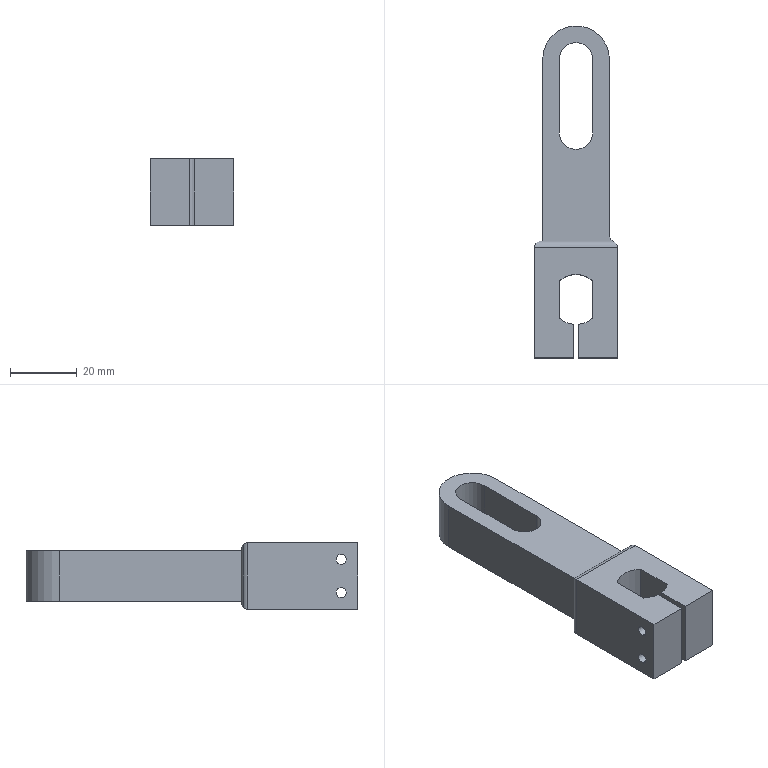Part | SolidWorks | features BaseBody 1 | 1 solid | 47 faces | box 25 x 99.5 x 20 mm | volume 28099 mm3 | cylinder 28 | plane 19 | commonest cylinder face diameters 4 x9 3 x8 6 x4 15 x3 10 x2 20 x2
STEP:
#1=CARTESIAN_POINT('',(10.5,17.5,2.));
#2=VERTEX_POINT('',#1);
#3=CARTESIAN_POINT('',(11.914,16.914,0.5858));
#4=VERTEX_POINT('',#3);
#5=CARTESIAN_POINT('',(10.5,17.5,2.));
#6=CARTESIAN_POINT('',(11.038,17.5,1.462));
#7=CARTESIAN_POINT('',(11.534,17.294,0.9659));
#8=CARTESIAN_POINT('',(11.914,16.914,0.5858));
#9=(BOUNDED_CURVE()B_SPLINE_CURVE(3,(#5,#6,#7,#8),.UNSPECIFIED.,.F.,.T.)B_SPLINE_CURVE_WITH_KNOTS((4,4),(1.571,2.356),.UNSPECIFIED.)CURVE()GEOMETRIC_REPRESENTATION_ITEM()RATIONAL_B_SPLINE_CURVE((1.,0.9493,0.9493,1.))REPRESENTATION_ITEM(''));
#10=EDGE_CURVE('',#2,#4,#9,.T.);
#11=ORIENTED_EDGE('',*,*,#10,.T.);
#12=CARTESIAN_POINT('',(-11.914,16.914,0.5858));
#13=VERTEX_POINT('',#12);
#14=CARTESIAN_POINT('',(0.,16.914,0.5858));
#15=DIRECTION('',(-1.,0.,0.));
#16=VECTOR('',#15,1000.);
#17=LINE('',#14,#16);
#18=EDGE_CURVE('',#4,#13,#17,.T.);
#19=ORIENTED_EDGE('',*,*,#18,.T.);
#20=CARTESIAN_POINT('',(-10.5,17.5,2.));
#21=VERTEX_POINT('',#20);
#22=CARTESIAN_POINT('',(-11.914,16.914,0.5858));
#23=CARTESIAN_POINT('',(-11.534,17.294,0.9659));
#24=CARTESIAN_POINT('',(-11.038,17.5,1.462));
#25=CARTESIAN_POINT('',(-10.5,17.5,2.));
#26=(BOUNDED_CURVE()B_SPLINE_CURVE(3,(#22,#23,#24,#25),.UNSPECIFIED.,.F.,.T.)B_SPLINE_CURVE_WITH_KNOTS((4,4),(0.7854,1.571),.UNSPECIFIED.)CURVE()GEOMETRIC_REPRESENTATION_ITEM()RATIONAL_B_SPLINE_CURVE((1.,0.9493,0.9493,1.))REPRESENTATION_ITEM(''));
#27=EDGE_CURVE('',#13,#21,#26,.T.);
#28=ORIENTED_EDGE('',*,*,#27,.T.);
#29=CARTESIAN_POINT('',(0.,17.5,2.));
#30=DIRECTION('',(1.,0.,0.));
#31=VECTOR('',#30,1000.);
#32=LINE('',#29,#31);
#33=EDGE_CURVE('',#21,#2,#32,.T.);
#34=ORIENTED_EDGE('',*,*,#33,.T.);
#35=EDGE_LOOP('',(#11,#19,#28,#34));
#36=FACE_OUTER_BOUND('',#35,.T.);
#37=CARTESIAN_POINT('',(0.,15.5,2.));
#38=DIRECTION('',(-1.,0.,0.));
#39=DIRECTION('',(0.,0.7071,-0.7071));
#40=AXIS2_PLACEMENT_3D('',#37,#38,#39);
#41=CYLINDRICAL_SURFACE('',#40,2.);
#42=ADVANCED_FACE('',(#36),#41,.T.);
#43=CARTESIAN_POINT('',(10.5,17.5,18.));
#44=VERTEX_POINT('',#43);
#45=CARTESIAN_POINT('',(11.914,16.914,19.414));
#46=VERTEX_POINT('',#45);
#47=CARTESIAN_POINT('',(10.5,17.5,18.));
#48=CARTESIAN_POINT('',(11.038,17.5,18.538));
#49=CARTESIAN_POINT('',(11.534,17.294,19.034));
#50=CARTESIAN_POINT('',(11.914,16.914,19.414));
#51=(BOUNDED_CURVE()B_SPLINE_CURVE(3,(#47,#48,#49,#50),.UNSPECIFIED.,.F.,.T.)B_SPLINE_CURVE_WITH_KNOTS((4,4),(1.571,2.356),.UNSPECIFIED.)CURVE()GEOMETRIC_REPRESENTATION_ITEM()RATIONAL_B_SPLINE_CURVE((1.,0.9493,0.9493,1.))REPRESENTATION_ITEM(''));
#52=EDGE_CURVE('',#44,#46,#51,.T.);
#53=ORIENTED_EDGE('',*,*,#52,.T.);
#54=CARTESIAN_POINT('',(11.914,16.914,0.));
#55=DIRECTION('',(0.,0.,-1.));
#56=VECTOR('',#55,1000.);
#57=LINE('',#54,#56);
#58=EDGE_CURVE('',#46,#4,#57,.T.);
#59=ORIENTED_EDGE('',*,*,#58,.T.);
#60=ORIENTED_EDGE('',*,*,#10,.F.);
#61=CARTESIAN_POINT('',(10.5,17.5,2.5));
#62=VERTEX_POINT('',#61);
#63=CARTESIAN_POINT('',(10.5,17.5,0.));
#64=DIRECTION('',(0.,0.,1.));
#65=VECTOR('',#64,1000.);
#66=LINE('',#63,#65);
#67=EDGE_CURVE('',#2,#62,#66,.T.);
#68=ORIENTED_EDGE('',*,*,#67,.T.);
#69=CARTESIAN_POINT('',(11.25,17.354,2.5));
#70=VERTEX_POINT('',#69);
#71=CARTESIAN_POINT('',(10.5,15.5,2.5));
#72=DIRECTION('',(0.,0.,-1.));
#73=DIRECTION('',(0.7071,0.7071,0.));
#74=AXIS2_PLACEMENT_3D('',#71,#72,#73);
#75=CIRCLE('',#74,2.);
#76=EDGE_CURVE('',#62,#70,#75,.T.);
#77=ORIENTED_EDGE('',*,*,#76,.T.);
#78=CARTESIAN_POINT('',(11.25,17.354,17.5));
#79=VERTEX_POINT('',#78);
#80=CARTESIAN_POINT('',(11.25,17.354,0.));
#81=DIRECTION('',(0.,0.,-1.));
#82=VECTOR('',#81,1000.);
#83=LINE('',#80,#82);
#84=EDGE_CURVE('',#79,#70,#83,.T.);
#85=ORIENTED_EDGE('',*,*,#84,.F.);
#86=CARTESIAN_POINT('',(10.5,17.5,17.5));
#87=VERTEX_POINT('',#86);
#88=CARTESIAN_POINT('',(10.5,15.5,17.5));
#89=DIRECTION('',(0.,0.,1.));
#90=DIRECTION('',(0.7071,0.7071,0.));
#91=AXIS2_PLACEMENT_3D('',#88,#89,#90);
#92=CIRCLE('',#91,2.);
#93=EDGE_CURVE('',#79,#87,#92,.T.);
#94=ORIENTED_EDGE('',*,*,#93,.T.);
#95=CARTESIAN_POINT('',(10.5,17.5,0.));
#96=DIRECTION('',(0.,0.,1.));
#97=VECTOR('',#96,1000.);
#98=LINE('',#95,#97);
#99=EDGE_CURVE('',#87,#44,#98,.T.);
#100=ORIENTED_EDGE('',*,*,#99,.T.);
#101=EDGE_LOOP('',(#53,#59,#60,#68,#77,#85,#94,#100));
#102=FACE_OUTER_BOUND('',#101,.T.);
#103=CARTESIAN_POINT('',(10.5,15.5,0.));
#104=DIRECTION('',(0.,0.,-1.));
#105=DIRECTION('',(0.7071,0.7071,0.));
#106=AXIS2_PLACEMENT_3D('',#103,#104,#105);
#107=CYLINDRICAL_SURFACE('',#106,2.);
#108=ADVANCED_FACE('',(#102),#107,.T.);
#109=CARTESIAN_POINT('',(-11.914,16.914,19.414));
#110=VERTEX_POINT('',#109);
#111=CARTESIAN_POINT('',(-10.5,17.5,18.));
#112=VERTEX_POINT('',#111);
#113=CARTESIAN_POINT('',(-11.914,16.914,19.414));
#114=CARTESIAN_POINT('',(-11.534,17.294,19.034));
#115=CARTESIAN_POINT('',(-11.038,17.5,18.538));
#116=CARTESIAN_POINT('',(-10.5,17.5,18.));
#117=(BOUNDED_CURVE()B_SPLINE_CURVE(3,(#113,#114,#115,#116),.UNSPECIFIED.,.F.,.T.)B_SPLINE_CURVE_WITH_KNOTS((4,4),(3.927,4.712),.UNSPECIFIED.)CURVE()GEOMETRIC_REPRESENTATION_ITEM()RATIONAL_B_SPLINE_CURVE((1.,0.9493,0.9493,1.))REPRESENTATION_ITEM(''));
#118=EDGE_CURVE('',#110,#112,#117,.T.);
#119=ORIENTED_EDGE('',*,*,#118,.F.);
#120=CARTESIAN_POINT('',(-0.9115,16.914,19.414));
#121=DIRECTION('',(1.,0.,0.));
#122=VECTOR('',#121,1000.);
#123=LINE('',#120,#122);
#124=EDGE_CURVE('',#110,#46,#123,.T.);
#125=ORIENTED_EDGE('',*,*,#124,.T.);
#126=ORIENTED_EDGE('',*,*,#52,.F.);
#127=CARTESIAN_POINT('',(-0.9115,17.5,18.));
#128=DIRECTION('',(-1.,0.,0.));
#129=VECTOR('',#128,1000.);
#130=LINE('',#127,#129);
#131=EDGE_CURVE('',#44,#112,#130,.T.);
#132=ORIENTED_EDGE('',*,*,#131,.T.);
#133=EDGE_LOOP('',(#119,#125,#126,#132));
#134=FACE_OUTER_BOUND('',#133,.T.);
#135=CARTESIAN_POINT('',(-0.9115,15.5,18.));
#136=DIRECTION('',(1.,0.,0.));
#137=DIRECTION('',(0.,0.7071,0.7071));
#138=AXIS2_PLACEMENT_3D('',#135,#136,#137);
#139=CYLINDRICAL_SURFACE('',#138,2.);
#140=ADVANCED_FACE('',(#134),#139,.T.);
#141=CARTESIAN_POINT('',(-12.5,15.5,20.));
#142=VERTEX_POINT('',#141);
#143=CARTESIAN_POINT('',(-12.5,15.5,20.));
#144=CARTESIAN_POINT('',(-12.5,16.038,20.));
#145=CARTESIAN_POINT('',(-12.294,16.534,19.794));
#146=CARTESIAN_POINT('',(-11.914,16.914,19.414));
#147=(BOUNDED_CURVE()B_SPLINE_CURVE(3,(#143,#144,#145,#146),.UNSPECIFIED.,.F.,.T.)B_SPLINE_CURVE_WITH_KNOTS((4,4),(3.142,3.927),.UNSPECIFIED.)CURVE()GEOMETRIC_REPRESENTATION_ITEM()RATIONAL_B_SPLINE_CURVE((1.,0.9493,0.9493,1.))REPRESENTATION_ITEM(''));
#148=EDGE_CURVE('',#142,#110,#147,.T.);
#149=ORIENTED_EDGE('',*,*,#148,.T.);
#150=CARTESIAN_POINT('',(-11.914,16.914,0.));
#151=DIRECTION('',(0.,0.,-1.));
#152=VECTOR('',#151,1000.);
#153=LINE('',#150,#152);
#154=EDGE_CURVE('',#110,#13,#153,.T.);
#155=ORIENTED_EDGE('',*,*,#154,.T.);
#156=CARTESIAN_POINT('',(-12.5,15.5,0.));
#157=VERTEX_POINT('',#156);
#158=CARTESIAN_POINT('',(-12.5,15.5,0.));
#159=CARTESIAN_POINT('',(-12.5,16.038,0.));
#160=CARTESIAN_POINT('',(-12.294,16.534,0.2057));
#161=CARTESIAN_POINT('',(-11.914,16.914,0.5858));
#162=(BOUNDED_CURVE()B_SPLINE_CURVE(3,(#158,#159,#160,#161),.UNSPECIFIED.,.F.,.T.)B_SPLINE_CURVE_WITH_KNOTS((4,4),(0.,0.7854),.UNSPECIFIED.)CURVE()GEOMETRIC_REPRESENTATION_ITEM()RATIONAL_B_SPLINE_CURVE((1.,0.9493,0.9493,1.))REPRESENTATION_ITEM(''));
#163=EDGE_CURVE('',#157,#13,#162,.T.);
#164=ORIENTED_EDGE('',*,*,#163,.F.);
#165=CARTESIAN_POINT('',(-12.5,15.5,0.));
#166=DIRECTION('',(0.,0.,1.));
#167=VECTOR('',#166,1000.);
#168=LINE('',#165,#167);
#169=EDGE_CURVE('',#157,#142,#168,.T.);
#170=ORIENTED_EDGE('',*,*,#169,.T.);
#171=EDGE_LOOP('',(#149,#155,#164,#170));
#172=FACE_OUTER_BOUND('',#171,.T.);
#173=CARTESIAN_POINT('',(-10.5,15.5,0.));
#174=DIRECTION('',(0.,0.,-1.));
#175=DIRECTION('',(-0.7071,0.7071,0.));
#176=AXIS2_PLACEMENT_3D('',#173,#174,#175);
#177=CYLINDRICAL_SURFACE('',#176,2.);
#178=ADVANCED_FACE('',(#172),#177,.T.);
#179=CARTESIAN_POINT('',(-10.,72.,17.5));
#180=VERTEX_POINT('',#179);
#181=CARTESIAN_POINT('',(7.071,79.071,17.5));
#182=VERTEX_POINT('',#181);
#183=CARTESIAN_POINT('',(0.,72.,17.5));
#184=DIRECTION('',(0.,0.,-1.));
#185=DIRECTION('',(0.7071,0.7071,0.));
#186=AXIS2_PLACEMENT_3D('',#183,#184,#185);
#187=CIRCLE('',#186,10.);
#188=EDGE_CURVE('',#180,#182,#187,.T.);
#189=ORIENTED_EDGE('',*,*,#188,.T.);
#190=CARTESIAN_POINT('',(7.071,79.071,2.5));
#191=VERTEX_POINT('',#190);
#192=CARTESIAN_POINT('',(7.071,79.071,0.));
#193=DIRECTION('',(0.,0.,-1.));
#194=VECTOR('',#193,1000.);
#195=LINE('',#192,#194);
#196=EDGE_CURVE('',#182,#191,#195,.T.);
#197=ORIENTED_EDGE('',*,*,#196,.T.);
#198=CARTESIAN_POINT('',(-10.,72.,2.5));
#199=VERTEX_POINT('',#198);
#200=CARTESIAN_POINT('',(0.,72.,2.5));
#201=DIRECTION('',(0.,0.,1.));
#202=DIRECTION('',(-0.7071,0.7071,0.));
#203=AXIS2_PLACEMENT_3D('',#200,#201,#202);
#204=CIRCLE('',#203,10.);
#205=EDGE_CURVE('',#191,#199,#204,.T.);
#206=ORIENTED_EDGE('',*,*,#205,.T.);
#207=CARTESIAN_POINT('',(-10.,72.,0.));
#208=DIRECTION('',(0.,0.,1.));
#209=VECTOR('',#208,1000.);
#210=LINE('',#207,#209);
#211=EDGE_CURVE('',#199,#180,#210,.T.);
#212=ORIENTED_EDGE('',*,*,#211,.T.);
#213=EDGE_LOOP('',(#189,#197,#206,#212));
#214=FACE_OUTER_BOUND('',#213,.T.);
#215=CARTESIAN_POINT('',(0.,72.,0.));
#216=DIRECTION('',(0.,0.,-1.));
#217=DIRECTION('',(0.7071,0.7071,0.));
#218=AXIS2_PLACEMENT_3D('',#215,#216,#217);
#219=CYLINDRICAL_SURFACE('',#218,10.);
#220=ADVANCED_FACE('',(#214),#219,.T.);
#221=CARTESIAN_POINT('',(8.5,-12.5,8.));
#222=VERTEX_POINT('',#221);
#223=CARTESIAN_POINT('',(8.5,-12.5,2.));
#224=VERTEX_POINT('',#223);
#225=CARTESIAN_POINT('',(8.5,-12.5,5.));
#226=DIRECTION('',(-1.,0.,0.));
#227=DIRECTION('',(0.,0.,1.));
#228=AXIS2_PLACEMENT_3D('',#225,#226,#227);
#229=CIRCLE('',#228,3.);
#230=EDGE_CURVE('',#222,#224,#229,.T.);
#231=ORIENTED_EDGE('',*,*,#230,.T.);
#232=CARTESIAN_POINT('',(12.5,-12.5,2.));
#233=VERTEX_POINT('',#232);
#234=CARTESIAN_POINT('',(12.5,-12.5,2.));
#235=DIRECTION('',(1.,0.,0.));
#236=VECTOR('',#235,1000.);
#237=LINE('',#234,#236);
#238=EDGE_CURVE('',#224,#233,#237,.T.);
#239=ORIENTED_EDGE('',*,*,#238,.T.);
#240=CARTESIAN_POINT('',(12.5,-12.5,8.));
#241=VERTEX_POINT('',#240);
#242=CARTESIAN_POINT('',(12.5,-12.5,5.));
#243=DIRECTION('',(-1.,0.,0.));
#244=DIRECTION('',(0.,0.,1.));
#245=AXIS2_PLACEMENT_3D('',#242,#243,#244);
#246=CIRCLE('',#245,3.);
#247=EDGE_CURVE('',#241,#233,#246,.T.);
#248=ORIENTED_EDGE('',*,*,#247,.F.);
#249=CARTESIAN_POINT('',(12.5,-12.5,8.));
#250=DIRECTION('',(1.,0.,0.));
#251=VECTOR('',#250,1000.);
#252=LINE('',#249,#251);
#253=EDGE_CURVE('',#222,#241,#252,.T.);
#254=ORIENTED_EDGE('',*,*,#253,.F.);
#255=EDGE_LOOP('',(#231,#239,#248,#254));
#256=FACE_OUTER_BOUND('',#255,.T.);
#257=CARTESIAN_POINT('',(12.5,-12.5,5.));
#258=DIRECTION('',(1.,0.,0.));
#259=DIRECTION('',(0.,0.,1.));
#260=AXIS2_PLACEMENT_3D('',#257,#258,#259);
#261=CYLINDRICAL_SURFACE('',#260,3.);
#262=ADVANCED_FACE('',(#256),#261,.F.);
#263=CARTESIAN_POINT('',(8.5,-12.5,18.));
#264=VERTEX_POINT('',#263);
#265=CARTESIAN_POINT('',(8.5,-12.5,12.));
#266=VERTEX_POINT('',#265);
#267=CARTESIAN_POINT('',(8.5,-12.5,15.));
#268=DIRECTION('',(-1.,0.,0.));
#269=DIRECTION('',(0.,0.,1.));
#270=AXIS2_PLACEMENT_3D('',#267,#268,#269);
#271=CIRCLE('',#270,3.);
#272=EDGE_CURVE('',#264,#266,#271,.T.);
#273=ORIENTED_EDGE('',*,*,#272,.T.);
#274=CARTESIAN_POINT('',(12.5,-12.5,12.));
#275=VERTEX_POINT('',#274);
#276=CARTESIAN_POINT('',(12.5,-12.5,12.));
#277=DIRECTION('',(1.,0.,0.));
#278=VECTOR('',#277,1000.);
#279=LINE('',#276,#278);
#280=EDGE_CURVE('',#266,#275,#279,.T.);
#281=ORIENTED_EDGE('',*,*,#280,.T.);
#282=CARTESIAN_POINT('',(12.5,-12.5,18.));
#283=VERTEX_POINT('',#282);
#284=CARTESIAN_POINT('',(12.5,-12.5,15.));
#285=DIRECTION('',(-1.,0.,0.));
#286=DIRECTION('',(0.,0.,1.));
#287=AXIS2_PLACEMENT_3D('',#284,#285,#286);
#288=CIRCLE('',#287,3.);
#289=EDGE_CURVE('',#283,#275,#288,.T.);
#290=ORIENTED_EDGE('',*,*,#289,.F.);
#291=CARTESIAN_POINT('',(12.5,-12.5,18.));
#292=DIRECTION('',(1.,0.,0.));
#293=VECTOR('',#292,1000.);
#294=LINE('',#291,#293);
#295=EDGE_CURVE('',#264,#283,#294,.T.);
#296=ORIENTED_EDGE('',*,*,#295,.F.);
#297=EDGE_LOOP('',(#273,#281,#290,#296));
#298=FACE_OUTER_BOUND('',#297,.T.);
#299=CARTESIAN_POINT('',(12.5,-12.5,15.));
#300=DIRECTION('',(1.,0.,0.));
#301=DIRECTION('',(0.,0.,1.));
#302=AXIS2_PLACEMENT_3D('',#299,#300,#301);
#303=CYLINDRICAL_SURFACE('',#302,3.);
#304=ADVANCED_FACE('',(#298),#303,.F.);
#305=CARTESIAN_POINT('',(8.5,-12.5,3.5));
#306=VERTEX_POINT('',#305);
#307=CARTESIAN_POINT('',(8.5,-12.5,6.5));
#308=VERTEX_POINT('',#307);
#309=CARTESIAN_POINT('',(8.5,-12.5,5.));
#310=DIRECTION('',(1.,0.,0.));
#311=DIRECTION('',(0.,0.,-1.));
#312=AXIS2_PLACEMENT_3D('',#309,#310,#311);
#313=CIRCLE('',#312,1.5);
#314=EDGE_CURVE('',#306,#308,#313,.T.);
#315=ORIENTED_EDGE('',*,*,#314,.T.);
#316=CARTESIAN_POINT('',(0.75,-12.5,6.5));
#317=VERTEX_POINT('',#316);
#318=CARTESIAN_POINT('',(-12.5,-12.5,6.5));
#319=DIRECTION('',(-1.,0.,0.));
#320=VECTOR('',#319,1000.);
#321=LINE('',#318,#320);
#322=EDGE_CURVE('',#308,#317,#321,.T.);
#323=ORIENTED_EDGE('',*,*,#322,.T.);
#324=CARTESIAN_POINT('',(0.75,-12.5,3.5));
#325=VERTEX_POINT('',#324);
#326=CARTESIAN_POINT('',(0.75,-12.5,5.));
#327=DIRECTION('',(1.,0.,0.));
#328=DIRECTION('',(0.,0.,-1.));
#329=AXIS2_PLACEMENT_3D('',#326,#327,#328);
#330=CIRCLE('',#329,1.5);
#331=EDGE_CURVE('',#325,#317,#330,.T.);
#332=ORIENTED_EDGE('',*,*,#331,.F.);
#333=CARTESIAN_POINT('',(-12.5,-12.5,3.5));
#334=DIRECTION('',(-1.,0.,0.));
#335=VECTOR('',#334,1000.);
#336=LINE('',#333,#335);
#337=EDGE_CURVE('',#306,#325,#336,.T.);
#338=ORIENTED_EDGE('',*,*,#337,.F.);
#339=EDGE_LOOP('',(#315,#323,#332,#338));
#340=FACE_OUTER_BOUND('',#339,.T.);
#341=CARTESIAN_POINT('',(-12.5,-12.5,5.));
#342=DIRECTION('',(-1.,0.,0.));
#343=DIRECTION('',(0.,0.,-1.));
#344=AXIS2_PLACEMENT_3D('',#341,#342,#343);
#345=CYLINDRICAL_SURFACE('',#344,1.5);
#346=ADVANCED_FACE('',(#340),#345,.F.);
#347=CARTESIAN_POINT('',(-0.75,-12.5,6.5));
#348=VERTEX_POINT('',#347);
#349=CARTESIAN_POINT('',(-0.75,-12.5,3.5));
#350=VERTEX_POINT('',#349);
#351=CARTESIAN_POINT('',(-0.75,-12.5,5.));
#352=DIRECTION('',(-1.,0.,0.));
#353=DIRECTION('',(0.,0.,-1.));
#354=AXIS2_PLACEMENT_3D('',#351,#352,#353);
#355=CIRCLE('',#354,1.5);
#356=EDGE_CURVE('',#348,#350,#355,.T.);
#357=ORIENTED_EDGE('',*,*,#356,.F.);
#358=CARTESIAN_POINT('',(-12.5,-12.5,6.5));
#359=VERTEX_POINT('',#358);
#360=CARTESIAN_POINT('',(-12.5,-12.5,6.5));
#361=DIRECTION('',(-1.,0.,0.));
#362=VECTOR('',#361,1000.);
#363=LINE('',#360,#362);
#364=EDGE_CURVE('',#348,#359,#363,.T.);
#365=ORIENTED_EDGE('',*,*,#364,.T.);
#366=CARTESIAN_POINT('',(-12.5,-12.5,3.5));
#367=VERTEX_POINT('',#366);
#368=CARTESIAN_POINT('',(-12.5,-12.5,5.));
#369=DIRECTION('',(1.,0.,0.));
#370=DIRECTION('',(0.,0.,-1.));
#371=AXIS2_PLACEMENT_3D('',#368,#369,#370);
#372=CIRCLE('',#371,1.5);
#373=EDGE_CURVE('',#367,#359,#372,.T.);
#374=ORIENTED_EDGE('',*,*,#373,.F.);
#375=CARTESIAN_POINT('',(-12.5,-12.5,3.5));
#376=DIRECTION('',(-1.,0.,0.));
#377=VECTOR('',#376,1000.);
#378=LINE('',#375,#377);
#379=EDGE_CURVE('',#350,#367,#378,.T.);
#380=ORIENTED_EDGE('',*,*,#379,.F.);
#381=EDGE_LOOP('',(#357,#365,#374,#380));
#382=FACE_OUTER_BOUND('',#381,.T.);
#383=CARTESIAN_POINT('',(-12.5,-12.5,5.));
#384=DIRECTION('',(-1.,0.,0.));
#385=DIRECTION('',(0.,0.,-1.));
#386=AXIS2_PLACEMENT_3D('',#383,#384,#385);
#387=CYLINDRICAL_SURFACE('',#386,1.5);
#388=ADVANCED_FACE('',(#382),#387,.F.);
#389=CARTESIAN_POINT('',(8.5,-12.5,13.5));
#390=VERTEX_POINT('',#389);
#391=CARTESIAN_POINT('',(8.5,-12.5,16.5));
#392=VERTEX_POINT('',#391);
#393=CARTESIAN_POINT('',(8.5,-12.5,15.));
#394=DIRECTION('',(1.,0.,0.));
#395=DIRECTION('',(0.,0.,-1.));
#396=AXIS2_PLACEMENT_3D('',#393,#394,#395);
#397=CIRCLE('',#396,1.5);
#398=EDGE_CURVE('',#390,#392,#397,.T.);
#399=ORIENTED_EDGE('',*,*,#398,.T.);
#400=CARTESIAN_POINT('',(0.75,-12.5,16.5));
#401=VERTEX_POINT('',#400);
#402=CARTESIAN_POINT('',(-12.5,-12.5,16.5));
#403=DIRECTION('',(-1.,0.,0.));
#404=VECTOR('',#403,1000.);
#405=LINE('',#402,#404);
#406=EDGE_CURVE('',#392,#401,#405,.T.);
#407=ORIENTED_EDGE('',*,*,#406,.T.);
#408=CARTESIAN_POINT('',(0.75,-12.5,13.5));
#409=VERTEX_POINT('',#408);
#410=CARTESIAN_POINT('',(0.75,-12.5,15.));
#411=DIRECTION('',(1.,0.,0.));
#412=DIRECTION('',(0.,0.,-1.));
#413=AXIS2_PLACEMENT_3D('',#410,#411,#412);
#414=CIRCLE('',#413,1.5);
#415=EDGE_CURVE('',#409,#401,#414,.T.);
#416=ORIENTED_EDGE('',*,*,#415,.F.);
#417=CARTESIAN_POINT('',(-12.5,-12.5,13.5));
#418=DIRECTION('',(-1.,0.,0.));
#419=VECTOR('',#418,1000.);
#420=LINE('',#417,#419);
#421=EDGE_CURVE('',#390,#409,#420,.T.);
#422=ORIENTED_EDGE('',*,*,#421,.F.);
#423=EDGE_LOOP('',(#399,#407,#416,#422));
#424=FACE_OUTER_BOUND('',#423,.T.);
#425=CARTESIAN_POINT('',(-12.5,-12.5,15.));
#426=DIRECTION('',(-1.,0.,0.));
#427=DIRECTION('',(0.,0.,-1.));
#428=AXIS2_PLACEMENT_3D('',#425,#426,#427);
#429=CYLINDRICAL_SURFACE('',#428,1.5);
#430=ADVANCED_FACE('',(#424),#429,.F.);
#431=CARTESIAN_POINT('',(-0.75,-12.5,16.5));
#432=VERTEX_POINT('',#431);
#433=CARTESIAN_POINT('',(-0.75,-12.5,13.5));
#434=VERTEX_POINT('',#433);
#435=CARTESIAN_POINT('',(-0.75,-12.5,15.));
#436=DIRECTION('',(-1.,0.,0.));
#437=DIRECTION('',(0.,0.,-1.));
#438=AXIS2_PLACEMENT_3D('',#435,#436,#437);
#439=CIRCLE('',#438,1.5);
#440=EDGE_CURVE('',#432,#434,#439,.T.);
#441=ORIENTED_EDGE('',*,*,#440,.F.);
#442=CARTESIAN_POINT('',(-12.5,-12.5,16.5));
#443=VERTEX_POINT('',#442);
#444=CARTESIAN_POINT('',(-12.5,-12.5,16.5));
#445=DIRECTION('',(-1.,0.,0.));
#446=VECTOR('',#445,1000.);
#447=LINE('',#444,#446);
#448=EDGE_CURVE('',#432,#443,#447,.T.);
#449=ORIENTED_EDGE('',*,*,#448,.T.);
#450=CARTESIAN_POINT('',(-12.5,-12.5,13.5));
#451=VERTEX_POINT('',#450);
#452=CARTESIAN_POINT('',(-12.5,-12.5,15.));
#453=DIRECTION('',(1.,0.,0.));
#454=DIRECTION('',(0.,0.,-1.));
#455=AXIS2_PLACEMENT_3D('',#452,#453,#454);
#456=CIRCLE('',#455,1.5);
#457=EDGE_CURVE('',#451,#443,#456,.T.);
#458=ORIENTED_EDGE('',*,*,#457,.F.);
#459=CARTESIAN_POINT('',(-12.5,-12.5,13.5));
#460=DIRECTION('',(-1.,0.,0.));
#461=VECTOR('',#460,1000.);
#462=LINE('',#459,#461);
#463=EDGE_CURVE('',#434,#451,#462,.T.);
#464=ORIENTED_EDGE('',*,*,#463,.F.);
#465=EDGE_LOOP('',(#441,#449,#458,#464));
#466=FACE_OUTER_BOUND('',#465,.T.);
#467=CARTESIAN_POINT('',(-12.5,-12.5,15.));
#468=DIRECTION('',(-1.,0.,0.));
#469=DIRECTION('',(0.,0.,-1.));
#470=AXIS2_PLACEMENT_3D('',#467,#468,#469);
#471=CYLINDRICAL_SURFACE('',#470,1.5);
#472=ADVANCED_FACE('',(#466),#471,.F.);
#473=CARTESIAN_POINT('',(10.,19.208,17.5));
#474=VERTEX_POINT('',#473);
#475=CARTESIAN_POINT('',(12.,19.208,17.5));
#476=DIRECTION('',(0.,0.,-1.));
#477=DIRECTION('',(1.,0.,0.));
#478=AXIS2_PLACEMENT_3D('',#475,#476,#477);
#479=CIRCLE('',#478,2.);
#480=EDGE_CURVE('',#79,#474,#479,.T.);
#481=ORIENTED_EDGE('',*,*,#480,.F.);
#482=ORIENTED_EDGE('',*,*,#84,.T.);
#483=CARTESIAN_POINT('',(10.,19.208,2.5));
#484=VERTEX_POINT('',#483);
#485=CARTESIAN_POINT('',(12.,19.208,2.5));
#486=DIRECTION('',(0.,0.,-1.));
#487=DIRECTION('',(1.,0.,0.));
#488=AXIS2_PLACEMENT_3D('',#485,#486,#487);
#489=CIRCLE('',#488,2.);
#490=EDGE_CURVE('',#70,#484,#489,.T.);
#491=ORIENTED_EDGE('',*,*,#490,.T.);
#492=CARTESIAN_POINT('',(10.,19.208,0.));
#493=DIRECTION('',(0.,0.,1.));
#494=VECTOR('',#493,1000.);
#495=LINE('',#492,#494);
#496=EDGE_CURVE('',#484,#474,#495,.T.);
#497=ORIENTED_EDGE('',*,*,#496,.T.);
#498=EDGE_LOOP('',(#481,#482,#491,#497));
#499=FACE_OUTER_BOUND('',#498,.T.);
#500=CARTESIAN_POINT('',(12.,19.208,0.));
#501=DIRECTION('',(0.,0.,-1.));
#502=DIRECTION('',(1.,0.,0.));
#503=AXIS2_PLACEMENT_3D('',#500,#501,#502);
#504=CYLINDRICAL_SURFACE('',#503,2.);
#505=ADVANCED_FACE('',(#499),#504,.F.);
#506=ORIENTED_EDGE('',*,*,#496,.F.);
#507=CARTESIAN_POINT('',(10.,72.,2.5));
#508=VERTEX_POINT('',#507);
#509=CARTESIAN_POINT('',(10.,17.5,2.5));
#510=DIRECTION('',(0.,1.,0.));
#511=VECTOR('',#510,1000.);
#512=LINE('',#509,#511);
#513=EDGE_CURVE('',#484,#508,#512,.T.);
#514=ORIENTED_EDGE('',*,*,#513,.T.);
#515=CARTESIAN_POINT('',(10.,72.,17.5));
#516=VERTEX_POINT('',#515);
#517=CARTESIAN_POINT('',(10.,72.,0.));
#518=DIRECTION('',(0.,0.,-1.));
#519=VECTOR('',#518,1000.);
#520=LINE('',#517,#519);
#521=EDGE_CURVE('',#516,#508,#520,.T.);
#522=ORIENTED_EDGE('',*,*,#521,.F.);
#523=CARTESIAN_POINT('',(10.,49.75,17.5));
#524=DIRECTION('',(0.,-1.,0.));
#525=VECTOR('',#524,1000.);
#526=LINE('',#523,#525);
#527=EDGE_CURVE('',#516,#474,#526,.T.);
#528=ORIENTED_EDGE('',*,*,#527,.T.);
#529=EDGE_LOOP('',(#506,#514,#522,#528));
#530=FACE_OUTER_BOUND('',#529,.T.);
#531=CARTESIAN_POINT('',(10.,17.5,0.));
#532=DIRECTION('',(1.,0.,0.));
#533=DIRECTION('',(0.,1.,0.));
#534=AXIS2_PLACEMENT_3D('',#531,#532,#533);
#535=PLANE('',#534);
#536=ADVANCED_FACE('',(#530),#535,.T.);
#537=ORIENTED_EDGE('',*,*,#457,.T.);
#538=CARTESIAN_POINT('',(-12.5,-12.5,15.));
#539=DIRECTION('',(1.,0.,0.));
#540=DIRECTION('',(0.,0.,-1.));
#541=AXIS2_PLACEMENT_3D('',#538,#539,#540);
#542=CIRCLE('',#541,1.5);
#543=EDGE_CURVE('',#443,#451,#542,.T.);
#544=ORIENTED_EDGE('',*,*,#543,.T.);
#545=EDGE_LOOP('',(#537,#544));
#546=FACE_BOUND('',#545,.T.);
#547=ORIENTED_EDGE('',*,*,#373,.T.);
#548=CARTESIAN_POINT('',(-12.5,-12.5,5.));
#549=DIRECTION('',(1.,0.,0.));
#550=DIRECTION('',(0.,0.,-1.));
#551=AXIS2_PLACEMENT_3D('',#548,#549,#550);
#552=CIRCLE('',#551,1.5);
#553=EDGE_CURVE('',#359,#367,#552,.T.);
#554=ORIENTED_EDGE('',*,*,#553,.T.);
#555=EDGE_LOOP('',(#547,#554));
#556=FACE_BOUND('',#555,.T.);
#557=ORIENTED_EDGE('',*,*,#169,.F.);
#558=CARTESIAN_POINT('',(-12.5,-17.5,0.));
#559=VERTEX_POINT('',#558);
#560=CARTESIAN_POINT('',(-12.5,17.5,0.));
#561=DIRECTION('',(0.,-1.,0.));
#562=VECTOR('',#561,1000.);
#563=LINE('',#560,#562);
#564=EDGE_CURVE('',#157,#559,#563,.T.);
#565=ORIENTED_EDGE('',*,*,#564,.T.);
#566=CARTESIAN_POINT('',(-12.5,-17.5,20.));
#567=VERTEX_POINT('',#566);
#568=CARTESIAN_POINT('',(-12.5,-17.5,0.));
#569=DIRECTION('',(0.,0.,1.));
#570=VECTOR('',#569,1000.);
#571=LINE('',#568,#570);
#572=EDGE_CURVE('',#559,#567,#571,.T.);
#573=ORIENTED_EDGE('',*,*,#572,.T.);
#574=CARTESIAN_POINT('',(-12.5,17.5,20.));
#575=DIRECTION('',(0.,-1.,0.));
#576=VECTOR('',#575,1000.);
#577=LINE('',#574,#576);
#578=EDGE_CURVE('',#142,#567,#577,.T.);
#579=ORIENTED_EDGE('',*,*,#578,.F.);
#580=EDGE_LOOP('',(#557,#565,#573,#579));
#581=FACE_OUTER_BOUND('',#580,.T.);
#582=CARTESIAN_POINT('',(-12.5,17.5,0.));
#583=DIRECTION('',(-1.,0.,0.));
#584=DIRECTION('',(0.,0.,1.));
#585=AXIS2_PLACEMENT_3D('',#582,#583,#584);
#586=PLANE('',#585);
#587=ADVANCED_FACE('',(#546,#556,#581),#586,.T.);
#588=CARTESIAN_POINT('',(12.5,15.5,0.));
#589=VERTEX_POINT('',#588);
#590=CARTESIAN_POINT('',(0.,15.5,0.));
#591=DIRECTION('',(-1.,0.,0.));
#592=VECTOR('',#591,1000.);
#593=LINE('',#590,#592);
#594=EDGE_CURVE('',#589,#157,#593,.T.);
#595=ORIENTED_EDGE('',*,*,#594,.F.);
#596=CARTESIAN_POINT('',(12.5,-17.5,0.));
#597=VERTEX_POINT('',#596);
#598=CARTESIAN_POINT('',(12.5,-17.5,0.));
#599=DIRECTION('',(0.,1.,0.));
#600=VECTOR('',#599,1000.);
#601=LINE('',#598,#600);
#602=EDGE_CURVE('',#597,#589,#601,.T.);
#603=ORIENTED_EDGE('',*,*,#602,.F.);
#604=CARTESIAN_POINT('',(0.75,-17.5,0.));
#605=VERTEX_POINT('',#604);
#606=CARTESIAN_POINT('',(-12.5,-17.5,0.));
#607=DIRECTION('',(1.,0.,0.));
#608=VECTOR('',#607,1000.);
#609=LINE('',#606,#608);
#610=EDGE_CURVE('',#605,#597,#609,.T.);
#611=ORIENTED_EDGE('',*,*,#610,.F.);
#612=CARTESIAN_POINT('',(0.75,-7.462,0.));
#613=VERTEX_POINT('',#612);
#614=CARTESIAN_POINT('',(0.75,21.144,0.));
#615=DIRECTION('',(0.,1.,0.));
#616=VECTOR('',#615,1000.);
#617=LINE('',#614,#616);
#618=EDGE_CURVE('',#605,#613,#617,.T.);
#619=ORIENTED_EDGE('',*,*,#618,.T.);
#620=CARTESIAN_POINT('',(5.,-5.59,0.));
#621=VERTEX_POINT('',#620);
#622=CARTESIAN_POINT('',(0.,0.,0.));
#623=DIRECTION('',(0.,0.,1.));
#624=DIRECTION('',(1.,0.,0.));
#625=AXIS2_PLACEMENT_3D('',#622,#623,#624);
#626=CIRCLE('',#625,7.5);
#627=EDGE_CURVE('',#613,#621,#626,.T.);
#628=ORIENTED_EDGE('',*,*,#627,.T.);
#629=CARTESIAN_POINT('',(5.,5.59,0.));
#630=VERTEX_POINT('',#629);
#631=CARTESIAN_POINT('',(5.,-5.59,0.));
#632=DIRECTION('',(0.,1.,0.));
#633=VECTOR('',#632,1000.);
#634=LINE('',#631,#633);
#635=EDGE_CURVE('',#621,#630,#634,.T.);
#636=ORIENTED_EDGE('',*,*,#635,.T.);
#637=CARTESIAN_POINT('',(-5.,5.59,0.));
#638=VERTEX_POINT('',#637);
#639=CARTESIAN_POINT('',(0.,0.,0.));
#640=DIRECTION('',(0.,0.,1.));
#641=DIRECTION('',(1.,0.,0.));
#642=AXIS2_PLACEMENT_3D('',#639,#640,#641);
#643=CIRCLE('',#642,7.5);
#644=EDGE_CURVE('',#630,#638,#643,.T.);
#645=ORIENTED_EDGE('',*,*,#644,.T.);
#646=CARTESIAN_POINT('',(-5.,-5.59,0.));
#647=VERTEX_POINT('',#646);
#648=CARTESIAN_POINT('',(-5.,5.59,0.));
#649=DIRECTION('',(0.,-1.,0.));
#650=VECTOR('',#649,1000.);
#651=LINE('',#648,#650);
#652=EDGE_CURVE('',#638,#647,#651,.T.);
#653=ORIENTED_EDGE('',*,*,#652,.T.);
#654=CARTESIAN_POINT('',(-0.75,-7.462,0.));
#655=VERTEX_POINT('',#654);
#656=CARTESIAN_POINT('',(0.,0.,0.));
#657=DIRECTION('',(0.,0.,1.));
#658=DIRECTION('',(1.,0.,0.));
#659=AXIS2_PLACEMENT_3D('',#656,#657,#658);
#660=CIRCLE('',#659,7.5);
#661=EDGE_CURVE('',#647,#655,#660,.T.);
#662=ORIENTED_EDGE('',*,*,#661,.T.);
#663=CARTESIAN_POINT('',(-0.75,-17.5,0.));
#664=VERTEX_POINT('',#663);
#665=CARTESIAN_POINT('',(-0.75,16.125,0.));
#666=DIRECTION('',(0.,-1.,0.));
#667=VECTOR('',#666,1000.);
#668=LINE('',#665,#667);
#669=EDGE_CURVE('',#655,#664,#668,.T.);
#670=ORIENTED_EDGE('',*,*,#669,.T.);
#671=CARTESIAN_POINT('',(-12.5,-17.5,0.));
#672=DIRECTION('',(1.,0.,0.));
#673=VECTOR('',#672,1000.);
#674=LINE('',#671,#673);
#675=EDGE_CURVE('',#559,#664,#674,.T.);
#676=ORIENTED_EDGE('',*,*,#675,.F.);
#677=ORIENTED_EDGE('',*,*,#564,.F.);
#678=EDGE_LOOP('',(#595,#603,#611,#619,#628,#636,#645,#653,#662,#670,#676,#677));
#679=FACE_OUTER_BOUND('',#678,.T.);
#680=CARTESIAN_POINT('',(0.,49.75,0.));
#681=DIRECTION('',(0.,0.,1.));
#682=DIRECTION('',(1.,0.,0.));
#683=AXIS2_PLACEMENT_3D('',#680,#681,#682);
#684=PLANE('',#683);
#685=ADVANCED_FACE('',(#679),#684,.F.);
#686=CARTESIAN_POINT('',(-10.,17.5,17.5));
#687=VERTEX_POINT('',#686);
#688=CARTESIAN_POINT('',(10.,17.5,17.5));
#689=DIRECTION('',(-1.,0.,0.));
#690=VECTOR('',#689,1000.);
#691=LINE('',#688,#690);
#692=EDGE_CURVE('',#87,#687,#691,.T.);
#693=ORIENTED_EDGE('',*,*,#692,.T.);
#694=CARTESIAN_POINT('',(-10.,17.5,2.5));
#695=VERTEX_POINT('',#694);
#696=CARTESIAN_POINT('',(-10.,17.5,0.));
#697=DIRECTION('',(0.,0.,1.));
#698=VECTOR('',#697,1000.);
#699=LINE('',#696,#698);
#700=EDGE_CURVE('',#695,#687,#699,.T.);
#701=ORIENTED_EDGE('',*,*,#700,.F.);
#702=CARTESIAN_POINT('',(5.,17.5,2.5));
#703=DIRECTION('',(1.,0.,0.));
#704=VECTOR('',#703,1000.);
#705=LINE('',#702,#704);
#706=EDGE_CURVE('',#695,#62,#705,.T.);
#707=ORIENTED_EDGE('',*,*,#706,.T.);
#708=ORIENTED_EDGE('',*,*,#67,.F.);
#709=ORIENTED_EDGE('',*,*,#33,.F.);
#710=CARTESIAN_POINT('',(-10.5,17.5,0.));
#711=DIRECTION('',(0.,0.,-1.));
#712=VECTOR('',#711,1000.);
#713=LINE('',#710,#712);
#714=EDGE_CURVE('',#112,#21,#713,.T.);
#715=ORIENTED_EDGE('',*,*,#714,.F.);
#716=ORIENTED_EDGE('',*,*,#131,.F.);
#717=ORIENTED_EDGE('',*,*,#99,.F.);
#718=EDGE_LOOP('',(#693,#701,#707,#708,#709,#715,#716,#717));
#719=FACE_OUTER_BOUND('',#718,.T.);
#720=CARTESIAN_POINT('',(0.,17.5,0.));
#721=DIRECTION('',(0.,1.,0.));
#722=DIRECTION('',(1.,0.,0.));
#723=AXIS2_PLACEMENT_3D('',#720,#721,#722);
#724=PLANE('',#723);
#725=ADVANCED_FACE('',(#719),#724,.T.);
#726=ORIENTED_EDGE('',*,*,#211,.F.);
#727=CARTESIAN_POINT('',(-10.,49.75,2.5));
#728=DIRECTION('',(0.,-1.,0.));
#729=VECTOR('',#728,1000.);
#730=LINE('',#727,#729);
#731=EDGE_CURVE('',#199,#695,#730,.T.);
#732=ORIENTED_EDGE('',*,*,#731,.T.);
#733=ORIENTED_EDGE('',*,*,#700,.T.);
#734=CARTESIAN_POINT('',(-10.,82.,17.5));
#735=DIRECTION('',(0.,1.,0.));
#736=VECTOR('',#735,1000.);
#737=LINE('',#734,#736);
#738=EDGE_CURVE('',#687,#180,#737,.T.);
#739=ORIENTED_EDGE('',*,*,#738,.T.);
#740=EDGE_LOOP('',(#726,#732,#733,#739));
#741=FACE_OUTER_BOUND('',#740,.T.);
#742=CARTESIAN_POINT('',(-10.,82.,0.));
#743=DIRECTION('',(-1.,0.,0.));
#744=DIRECTION('',(0.,1.,0.));
#745=AXIS2_PLACEMENT_3D('',#742,#743,#744);
#746=PLANE('',#745);
#747=ADVANCED_FACE('',(#741),#746,.T.);
#748=CARTESIAN_POINT('',(5.,72.,2.5));
#749=VERTEX_POINT('',#748);
#750=CARTESIAN_POINT('',(5.,50.,2.5));
#751=VERTEX_POINT('',#750);
#752=CARTESIAN_POINT('',(5.,44.75,2.5));
#753=DIRECTION('',(0.,-1.,0.));
#754=VECTOR('',#753,1000.);
#755=LINE('',#752,#754);
#756=EDGE_CURVE('',#749,#751,#755,.T.);
#757=ORIENTED_EDGE('',*,*,#756,.F.);
#758=CARTESIAN_POINT('',(-5.,72.,2.5));
#759=VERTEX_POINT('',#758);
#760=CARTESIAN_POINT('',(0.,72.,2.5));
#761=DIRECTION('',(0.,0.,-1.));
#762=DIRECTION('',(1.,0.,0.));
#763=AXIS2_PLACEMENT_3D('',#760,#761,#762);
#764=CIRCLE('',#763,5.);
#765=EDGE_CURVE('',#759,#749,#764,.T.);
#766=ORIENTED_EDGE('',*,*,#765,.F.);
#767=CARTESIAN_POINT('',(-5.,50.,2.5));
#768=VERTEX_POINT('',#767);
#769=CARTESIAN_POINT('',(-5.,33.75,2.5));
#770=DIRECTION('',(0.,1.,0.));
#771=VECTOR('',#770,1000.);
#772=LINE('',#769,#771);
#773=EDGE_CURVE('',#768,#759,#772,.T.);
#774=ORIENTED_EDGE('',*,*,#773,.F.);
#775=CARTESIAN_POINT('',(0.,50.,2.5));
#776=DIRECTION('',(0.,0.,-1.));
#777=DIRECTION('',(1.,0.,0.));
#778=AXIS2_PLACEMENT_3D('',#775,#776,#777);
#779=CIRCLE('',#778,5.);
#780=EDGE_CURVE('',#751,#768,#779,.T.);
#781=ORIENTED_EDGE('',*,*,#780,.F.);
#782=EDGE_LOOP('',(#757,#766,#774,#781));
#783=FACE_BOUND('',#782,.T.);
#784=CARTESIAN_POINT('',(0.,72.,2.5));
#785=DIRECTION('',(0.,0.,1.));
#786=DIRECTION('',(-0.7071,0.7071,0.));
#787=AXIS2_PLACEMENT_3D('',#784,#785,#786);
#788=CIRCLE('',#787,10.);
#789=EDGE_CURVE('',#508,#191,#788,.T.);
#790=ORIENTED_EDGE('',*,*,#789,.F.);
#791=ORIENTED_EDGE('',*,*,#513,.F.);
#792=ORIENTED_EDGE('',*,*,#490,.F.);
#793=ORIENTED_EDGE('',*,*,#76,.F.);
#794=ORIENTED_EDGE('',*,*,#706,.F.);
#795=ORIENTED_EDGE('',*,*,#731,.F.);
#796=ORIENTED_EDGE('',*,*,#205,.F.);
#797=EDGE_LOOP('',(#790,#791,#792,#793,#794,#795,#796));
#798=FACE_OUTER_BOUND('',#797,.T.);
#799=CARTESIAN_POINT('',(10.,17.5,2.5));
#800=DIRECTION('',(0.,0.,1.));
#801=DIRECTION('',(0.,-1.,0.));
#802=AXIS2_PLACEMENT_3D('',#799,#800,#801);
#803=PLANE('',#802);
#804=ADVANCED_FACE('',(#783,#798),#803,.F.);
#805=CARTESIAN_POINT('',(5.,50.,17.5));
#806=VERTEX_POINT('',#805);
#807=CARTESIAN_POINT('',(5.,72.,17.5));
#808=VERTEX_POINT('',#807);
#809=CARTESIAN_POINT('',(5.,77.,17.5));
#810=DIRECTION('',(0.,1.,0.));
#811=VECTOR('',#810,1000.);
#812=LINE('',#809,#811);
#813=EDGE_CURVE('',#806,#808,#812,.T.);
#814=ORIENTED_EDGE('',*,*,#813,.F.);
#815=CARTESIAN_POINT('',(-5.,50.,17.5));
#816=VERTEX_POINT('',#815);
#817=CARTESIAN_POINT('',(0.,50.,17.5));
#818=DIRECTION('',(0.,0.,1.));
#819=DIRECTION('',(1.,0.,0.));
#820=AXIS2_PLACEMENT_3D('',#817,#818,#819);
#821=CIRCLE('',#820,5.);
#822=EDGE_CURVE('',#816,#806,#821,.T.);
#823=ORIENTED_EDGE('',*,*,#822,.F.);
#824=CARTESIAN_POINT('',(-5.,72.,17.5));
#825=VERTEX_POINT('',#824);
#826=CARTESIAN_POINT('',(-5.,66.,17.5));
#827=DIRECTION('',(0.,-1.,0.));
#828=VECTOR('',#827,1000.);
#829=LINE('',#826,#828);
#830=EDGE_CURVE('',#825,#816,#829,.T.);
#831=ORIENTED_EDGE('',*,*,#830,.F.);
#832=CARTESIAN_POINT('',(0.,72.,17.5));
#833=DIRECTION('',(0.,0.,1.));
#834=DIRECTION('',(1.,0.,0.));
#835=AXIS2_PLACEMENT_3D('',#832,#833,#834);
#836=CIRCLE('',#835,5.);
#837=EDGE_CURVE('',#808,#825,#836,.T.);
#838=ORIENTED_EDGE('',*,*,#837,.F.);
#839=EDGE_LOOP('',(#814,#823,#831,#838));
#840=FACE_BOUND('',#839,.T.);
#841=ORIENTED_EDGE('',*,*,#188,.F.);
#842=ORIENTED_EDGE('',*,*,#738,.F.);
#843=ORIENTED_EDGE('',*,*,#692,.F.);
#844=ORIENTED_EDGE('',*,*,#93,.F.);
#845=ORIENTED_EDGE('',*,*,#480,.T.);
#846=ORIENTED_EDGE('',*,*,#527,.F.);
#847=CARTESIAN_POINT('',(0.,72.,17.5));
#848=DIRECTION('',(0.,0.,-1.));
#849=DIRECTION('',(0.7071,0.7071,0.));
#850=AXIS2_PLACEMENT_3D('',#847,#848,#849);
#851=CIRCLE('',#850,10.);
#852=EDGE_CURVE('',#182,#516,#851,.T.);
#853=ORIENTED_EDGE('',*,*,#852,.F.);
#854=EDGE_LOOP('',(#841,#842,#843,#844,#845,#846,#853));
#855=FACE_OUTER_BOUND('',#854,.T.);
#856=CARTESIAN_POINT('',(10.,82.,17.5));
#857=DIRECTION('',(0.,0.,-1.));
#858=DIRECTION('',(-1.,0.,0.));
#859=AXIS2_PLACEMENT_3D('',#856,#857,#858);
#860=PLANE('',#859);
#861=ADVANCED_FACE('',(#840,#855),#860,.F.);
#862=ORIENTED_EDGE('',*,*,#652,.F.);
#863=CARTESIAN_POINT('',(-5.,5.59,20.));
#864=VERTEX_POINT('',#863);
#865=CARTESIAN_POINT('',(-5.,5.59,20.));
#866=DIRECTION('',(0.,0.,-1.));
#867=VECTOR('',#866,1000.);
#868=LINE('',#865,#867);
#869=EDGE_CURVE('',#864,#638,#868,.T.);
#870=ORIENTED_EDGE('',*,*,#869,.F.);
#871=CARTESIAN_POINT('',(-5.,-5.59,20.));
#872=VERTEX_POINT('',#871);
#873=CARTESIAN_POINT('',(-5.,5.59,20.));
#874=DIRECTION('',(0.,1.,0.));
#875=VECTOR('',#874,1000.);
#876=LINE('',#873,#875);
#877=EDGE_CURVE('',#872,#864,#876,.T.);
#878=ORIENTED_EDGE('',*,*,#877,.F.);
#879=CARTESIAN_POINT('',(-5.,-5.59,20.));
#880=DIRECTION('',(0.,0.,1.));
#881=VECTOR('',#880,1000.);
#882=LINE('',#879,#881);
#883=EDGE_CURVE('',#647,#872,#882,.T.);
#884=ORIENTED_EDGE('',*,*,#883,.F.);
#885=EDGE_LOOP('',(#862,#870,#878,#884));
#886=FACE_OUTER_BOUND('',#885,.T.);
#887=CARTESIAN_POINT('',(-5.,-5.59,0.));
#888=DIRECTION('',(1.,0.,0.));
#889=DIRECTION('',(0.,-1.,0.));
#890=AXIS2_PLACEMENT_3D('',#887,#888,#889);
#891=PLANE('',#890);
#892=ADVANCED_FACE('',(#886),#891,.T.);
#893=ORIENTED_EDGE('',*,*,#635,.F.);
#894=CARTESIAN_POINT('',(5.,-5.59,20.));
#895=VERTEX_POINT('',#894);
#896=CARTESIAN_POINT('',(5.,-5.59,20.));
#897=DIRECTION('',(0.,0.,-1.));
#898=VECTOR('',#897,1000.);
#899=LINE('',#896,#898);
#900=EDGE_CURVE('',#895,#621,#899,.T.);
#901=ORIENTED_EDGE('',*,*,#900,.F.);
#902=CARTESIAN_POINT('',(5.,5.59,20.));
#903=VERTEX_POINT('',#902);
#904=CARTESIAN_POINT('',(5.,-5.59,20.));
#905=DIRECTION('',(0.,-1.,0.));
#906=VECTOR('',#905,1000.);
#907=LINE('',#904,#906);
#908=EDGE_CURVE('',#903,#895,#907,.T.);
#909=ORIENTED_EDGE('',*,*,#908,.F.);
#910=CARTESIAN_POINT('',(5.,5.59,20.));
#911=DIRECTION('',(0.,0.,1.));
#912=VECTOR('',#911,1000.);
#913=LINE('',#910,#912);
#914=EDGE_CURVE('',#630,#903,#913,.T.);
#915=ORIENTED_EDGE('',*,*,#914,.F.);
#916=EDGE_LOOP('',(#893,#901,#909,#915));
#917=FACE_OUTER_BOUND('',#916,.T.);
#918=CARTESIAN_POINT('',(5.,5.59,0.));
#919=DIRECTION('',(-1.,0.,0.));
#920=DIRECTION('',(0.,0.,1.));
#921=AXIS2_PLACEMENT_3D('',#918,#919,#920);
#922=PLANE('',#921);
#923=ADVANCED_FACE('',(#917),#922,.T.);
#924=ORIENTED_EDGE('',*,*,#900,.T.);
#925=ORIENTED_EDGE('',*,*,#627,.F.);
#926=CARTESIAN_POINT('',(0.75,-7.462,20.));
#927=VERTEX_POINT('',#926);
#928=CARTESIAN_POINT('',(0.75,-7.462,20.));
#929=DIRECTION('',(0.,0.,-1.));
#930=VECTOR('',#929,1000.);
#931=LINE('',#928,#930);
#932=EDGE_CURVE('',#927,#613,#931,.T.);
#933=ORIENTED_EDGE('',*,*,#932,.F.);
#934=CARTESIAN_POINT('',(0.,0.,20.));
#935=DIRECTION('',(0.,0.,-1.));
#936=DIRECTION('',(1.,0.,0.));
#937=AXIS2_PLACEMENT_3D('',#934,#935,#936);
#938=CIRCLE('',#937,7.5);
#939=EDGE_CURVE('',#895,#927,#938,.T.);
#940=ORIENTED_EDGE('',*,*,#939,.F.);
#941=EDGE_LOOP('',(#924,#925,#933,#940));
#942=FACE_OUTER_BOUND('',#941,.T.);
#943=CARTESIAN_POINT('',(0.,0.,20.));
#944=DIRECTION('',(0.,0.,1.));
#945=DIRECTION('',(1.,0.,0.));
#946=AXIS2_PLACEMENT_3D('',#943,#944,#945);
#947=CYLINDRICAL_SURFACE('',#946,7.5);
#948=ADVANCED_FACE('',(#942),#947,.F.);
#949=ORIENTED_EDGE('',*,*,#869,.T.);
#950=ORIENTED_EDGE('',*,*,#644,.F.);
#951=ORIENTED_EDGE('',*,*,#914,.T.);
#952=CARTESIAN_POINT('',(0.,0.,20.));
#953=DIRECTION('',(0.,0.,-1.));
#954=DIRECTION('',(1.,0.,0.));
#955=AXIS2_PLACEMENT_3D('',#952,#953,#954);
#956=CIRCLE('',#955,7.5);
#957=EDGE_CURVE('',#864,#903,#956,.T.);
#958=ORIENTED_EDGE('',*,*,#957,.F.);
#959=EDGE_LOOP('',(#949,#950,#951,#958));
#960=FACE_OUTER_BOUND('',#959,.T.);
#961=CARTESIAN_POINT('',(0.,0.,20.));
#962=DIRECTION('',(0.,0.,1.));
#963=DIRECTION('',(1.,0.,0.));
#964=AXIS2_PLACEMENT_3D('',#961,#962,#963);
#965=CYLINDRICAL_SURFACE('',#964,7.5);
#966=ADVANCED_FACE('',(#960),#965,.F.);
#967=ORIENTED_EDGE('',*,*,#883,.T.);
#968=CARTESIAN_POINT('',(-0.75,-7.462,20.));
#969=VERTEX_POINT('',#968);
#970=CARTESIAN_POINT('',(0.,0.,20.));
#971=DIRECTION('',(0.,0.,-1.));
#972=DIRECTION('',(1.,0.,0.));
#973=AXIS2_PLACEMENT_3D('',#970,#971,#972);
#974=CIRCLE('',#973,7.5);
#975=EDGE_CURVE('',#969,#872,#974,.T.);
#976=ORIENTED_EDGE('',*,*,#975,.F.);
#977=CARTESIAN_POINT('',(-0.75,-7.462,20.));
#978=DIRECTION('',(0.,0.,-1.));
#979=VECTOR('',#978,1000.);
#980=LINE('',#977,#979);
#981=EDGE_CURVE('',#969,#655,#980,.T.);
#982=ORIENTED_EDGE('',*,*,#981,.T.);
#983=ORIENTED_EDGE('',*,*,#661,.F.);
#984=EDGE_LOOP('',(#967,#976,#982,#983));
#985=FACE_OUTER_BOUND('',#984,.T.);
#986=CARTESIAN_POINT('',(0.,0.,20.));
#987=DIRECTION('',(0.,0.,1.));
#988=DIRECTION('',(1.,0.,0.));
#989=AXIS2_PLACEMENT_3D('',#986,#987,#988);
#990=CYLINDRICAL_SURFACE('',#989,7.5);
#991=ADVANCED_FACE('',(#985),#990,.F.);
#992=ORIENTED_EDGE('',*,*,#314,.F.);
#993=CARTESIAN_POINT('',(8.5,-12.5,5.));
#994=DIRECTION('',(1.,0.,0.));
#995=DIRECTION('',(0.,0.,-1.));
#996=AXIS2_PLACEMENT_3D('',#993,#994,#995);
#997=CIRCLE('',#996,1.5);
#998=EDGE_CURVE('',#308,#306,#997,.T.);
#999=ORIENTED_EDGE('',*,*,#998,.F.);
#1000=EDGE_LOOP('',(#992,#999));
#1001=FACE_BOUND('',#1000,.T.);
#1002=ORIENTED_EDGE('',*,*,#230,.F.);
#1003=CARTESIAN_POINT('',(8.5,-12.5,5.));
#1004=DIRECTION('',(-1.,0.,0.));
#1005=DIRECTION('',(0.,0.,1.));
#1006=AXIS2_PLACEMENT_3D('',#1003,#1004,#1005);
#1007=CIRCLE('',#1006,3.);
#1008=EDGE_CURVE('',#224,#222,#1007,.T.);
#1009=ORIENTED_EDGE('',*,*,#1008,.F.);
#1010=EDGE_LOOP('',(#1002,#1009));
#1011=FACE_OUTER_BOUND('',#1010,.T.);
#1012=CARTESIAN_POINT('',(8.5,-12.5,5.));
#1013=DIRECTION('',(-1.,0.,0.));
#1014=DIRECTION('',(0.,1.,0.));
#1015=AXIS2_PLACEMENT_3D('',#1012,#1013,#1014);
#1016=PLANE('',#1015);
#1017=ADVANCED_FACE('',(#1001,#1011),#1016,.F.);
#1018=ORIENTED_EDGE('',*,*,#398,.F.);
#1019=CARTESIAN_POINT('',(8.5,-12.5,15.));
#1020=DIRECTION('',(1.,0.,0.));
#1021=DIRECTION('',(0.,0.,-1.));
#1022=AXIS2_PLACEMENT_3D('',#1019,#1020,#1021);
#1023=CIRCLE('',#1022,1.5);
#1024=EDGE_CURVE('',#392,#390,#1023,.T.);
#1025=ORIENTED_EDGE('',*,*,#1024,.F.);
#1026=EDGE_LOOP('',(#1018,#1025));
#1027=FACE_BOUND('',#1026,.T.);
#1028=ORIENTED_EDGE('',*,*,#272,.F.);
#1029=CARTESIAN_POINT('',(8.5,-12.5,15.));
#1030=DIRECTION('',(-1.,0.,0.));
#1031=DIRECTION('',(0.,0.,1.));
#1032=AXIS2_PLACEMENT_3D('',#1029,#1030,#1031);
#1033=CIRCLE('',#1032,3.);
#1034=EDGE_CURVE('',#266,#264,#1033,.T.);
#1035=ORIENTED_EDGE('',*,*,#1034,.F.);
#1036=EDGE_LOOP('',(#1028,#1035));
#1037=FACE_OUTER_BOUND('',#1036,.T.);
#1038=CARTESIAN_POINT('',(8.5,-12.5,15.));
#1039=DIRECTION('',(-1.,0.,0.));
#1040=DIRECTION('',(0.,1.,0.));
#1041=AXIS2_PLACEMENT_3D('',#1038,#1039,#1040);
#1042=PLANE('',#1041);
#1043=ADVANCED_FACE('',(#1027,#1037),#1042,.F.);
#1044=ORIENTED_EDGE('',*,*,#773,.T.);
#1045=CARTESIAN_POINT('',(-5.,72.,20.));
#1046=DIRECTION('',(0.,0.,-1.));
#1047=VECTOR('',#1046,1000.);
#1048=LINE('',#1045,#1047);
#1049=EDGE_CURVE('',#825,#759,#1048,.T.);
#1050=ORIENTED_EDGE('',*,*,#1049,.F.);
#1051=ORIENTED_EDGE('',*,*,#830,.T.);
#1052=CARTESIAN_POINT('',(-5.,50.,20.));
#1053=DIRECTION('',(0.,0.,-1.));
#1054=VECTOR('',#1053,1000.);
#1055=LINE('',#1052,#1054);
#1056=EDGE_CURVE('',#816,#768,#1055,.T.);
#1057=ORIENTED_EDGE('',*,*,#1056,.T.);
#1058=EDGE_LOOP('',(#1044,#1050,#1051,#1057));
#1059=FACE_OUTER_BOUND('',#1058,.T.);
#1060=CARTESIAN_POINT('',(-5.,50.,20.));
#1061=DIRECTION('',(-1.,0.,0.));
#1062=DIRECTION('',(0.,1.,0.));
#1063=AXIS2_PLACEMENT_3D('',#1060,#1061,#1062);
#1064=PLANE('',#1063);
#1065=ADVANCED_FACE('',(#1059),#1064,.F.);
#1066=ORIENTED_EDGE('',*,*,#765,.T.);
#1067=CARTESIAN_POINT('',(5.,72.,20.));
#1068=DIRECTION('',(0.,0.,-1.));
#1069=VECTOR('',#1068,1000.);
#1070=LINE('',#1067,#1069);
#1071=EDGE_CURVE('',#808,#749,#1070,.T.);
#1072=ORIENTED_EDGE('',*,*,#1071,.F.);
#1073=ORIENTED_EDGE('',*,*,#837,.T.);
#1074=ORIENTED_EDGE('',*,*,#1049,.T.);
#1075=EDGE_LOOP('',(#1066,#1072,#1073,#1074));
#1076=FACE_OUTER_BOUND('',#1075,.T.);
#1077=CARTESIAN_POINT('',(0.,72.,20.));
#1078=DIRECTION('',(0.,0.,1.));
#1079=DIRECTION('',(1.,0.,0.));
#1080=AXIS2_PLACEMENT_3D('',#1077,#1078,#1079);
#1081=CYLINDRICAL_SURFACE('',#1080,5.);
#1082=ADVANCED_FACE('',(#1076),#1081,.F.);
#1083=ORIENTED_EDGE('',*,*,#756,.T.);
#1084=CARTESIAN_POINT('',(5.,50.,20.));
#1085=DIRECTION('',(0.,0.,-1.));
#1086=VECTOR('',#1085,1000.);
#1087=LINE('',#1084,#1086);
#1088=EDGE_CURVE('',#806,#751,#1087,.T.);
#1089=ORIENTED_EDGE('',*,*,#1088,.F.);
#1090=ORIENTED_EDGE('',*,*,#813,.T.);
#1091=ORIENTED_EDGE('',*,*,#1071,.T.);
#1092=EDGE_LOOP('',(#1083,#1089,#1090,#1091));
#1093=FACE_OUTER_BOUND('',#1092,.T.);
#1094=CARTESIAN_POINT('',(5.,72.,20.));
#1095=DIRECTION('',(1.,0.,0.));
#1096=DIRECTION('',(0.,1.,0.));
#1097=AXIS2_PLACEMENT_3D('',#1094,#1095,#1096);
#1098=PLANE('',#1097);
#1099=ADVANCED_FACE('',(#1093),#1098,.F.);
#1100=ORIENTED_EDGE('',*,*,#780,.T.);
#1101=ORIENTED_EDGE('',*,*,#1056,.F.);
#1102=ORIENTED_EDGE('',*,*,#822,.T.);
#1103=ORIENTED_EDGE('',*,*,#1088,.T.);
#1104=EDGE_LOOP('',(#1100,#1101,#1102,#1103));
#1105=FACE_OUTER_BOUND('',#1104,.T.);
#1106=CARTESIAN_POINT('',(0.,50.,20.));
#1107=DIRECTION('',(0.,0.,1.));
#1108=DIRECTION('',(1.,0.,0.));
#1109=AXIS2_PLACEMENT_3D('',#1106,#1107,#1108);
#1110=CYLINDRICAL_SURFACE('',#1109,5.);
#1111=ADVANCED_FACE('',(#1105),#1110,.F.);
#1112=CARTESIAN_POINT('',(-0.75,-12.5,5.));
#1113=DIRECTION('',(-1.,0.,0.));
#1114=DIRECTION('',(0.,0.,-1.));
#1115=AXIS2_PLACEMENT_3D('',#1112,#1113,#1114);
#1116=CIRCLE('',#1115,1.5);
#1117=EDGE_CURVE('',#350,#348,#1116,.T.);
#1118=ORIENTED_EDGE('',*,*,#1117,.T.);
#1119=ORIENTED_EDGE('',*,*,#356,.T.);
#1120=EDGE_LOOP('',(#1118,#1119));
#1121=FACE_BOUND('',#1120,.T.);
#1122=CARTESIAN_POINT('',(-0.75,-12.5,15.));
#1123=DIRECTION('',(-1.,0.,0.));
#1124=DIRECTION('',(0.,0.,-1.));
#1125=AXIS2_PLACEMENT_3D('',#1122,#1123,#1124);
#1126=CIRCLE('',#1125,1.5);
#1127=EDGE_CURVE('',#434,#432,#1126,.T.);
#1128=ORIENTED_EDGE('',*,*,#1127,.T.);
#1129=ORIENTED_EDGE('',*,*,#440,.T.);
#1130=EDGE_LOOP('',(#1128,#1129));
#1131=FACE_BOUND('',#1130,.T.);
#1132=ORIENTED_EDGE('',*,*,#669,.F.);
#1133=ORIENTED_EDGE('',*,*,#981,.F.);
#1134=CARTESIAN_POINT('',(-0.75,-17.5,20.));
#1135=VERTEX_POINT('',#1134);
#1136=CARTESIAN_POINT('',(-0.75,-9.661,20.));
#1137=DIRECTION('',(0.,1.,0.));
#1138=VECTOR('',#1137,1000.);
#1139=LINE('',#1136,#1138);
#1140=EDGE_CURVE('',#1135,#969,#1139,.T.);
#1141=ORIENTED_EDGE('',*,*,#1140,.F.);
#1142=CARTESIAN_POINT('',(-0.75,-17.5,10.));
#1143=DIRECTION('',(0.,0.,1.));
#1144=VECTOR('',#1143,1000.);
#1145=LINE('',#1142,#1144);
#1146=EDGE_CURVE('',#664,#1135,#1145,.T.);
#1147=ORIENTED_EDGE('',*,*,#1146,.F.);
#1148=EDGE_LOOP('',(#1132,#1133,#1141,#1147));
#1149=FACE_OUTER_BOUND('',#1148,.T.);
#1150=CARTESIAN_POINT('',(-0.75,-17.5,20.));
#1151=DIRECTION('',(-1.,0.,0.));
#1152=DIRECTION('',(0.,0.,1.));
#1153=AXIS2_PLACEMENT_3D('',#1150,#1151,#1152);
#1154=PLANE('',#1153);
#1155=ADVANCED_FACE('',(#1121,#1131,#1149),#1154,.F.);
#1156=ORIENTED_EDGE('',*,*,#331,.T.);
#1157=CARTESIAN_POINT('',(0.75,-12.5,5.));
#1158=DIRECTION('',(1.,0.,0.));
#1159=DIRECTION('',(0.,0.,-1.));
#1160=AXIS2_PLACEMENT_3D('',#1157,#1158,#1159);
#1161=CIRCLE('',#1160,1.5);
#1162=EDGE_CURVE('',#317,#325,#1161,.T.);
#1163=ORIENTED_EDGE('',*,*,#1162,.T.);
#1164=EDGE_LOOP('',(#1156,#1163));
#1165=FACE_BOUND('',#1164,.T.);
#1166=ORIENTED_EDGE('',*,*,#415,.T.);
#1167=CARTESIAN_POINT('',(0.75,-12.5,15.));
#1168=DIRECTION('',(1.,0.,0.));
#1169=DIRECTION('',(0.,0.,-1.));
#1170=AXIS2_PLACEMENT_3D('',#1167,#1168,#1169);
#1171=CIRCLE('',#1170,1.5);
#1172=EDGE_CURVE('',#401,#409,#1171,.T.);
#1173=ORIENTED_EDGE('',*,*,#1172,.T.);
#1174=EDGE_LOOP('',(#1166,#1173));
#1175=FACE_BOUND('',#1174,.T.);
#1176=ORIENTED_EDGE('',*,*,#618,.F.);
#1177=CARTESIAN_POINT('',(0.75,-17.5,20.));
#1178=VERTEX_POINT('',#1177);
#1179=CARTESIAN_POINT('',(0.75,-17.5,10.));
#1180=DIRECTION('',(0.,0.,-1.));
#1181=VECTOR('',#1180,1000.);
#1182=LINE('',#1179,#1181);
#1183=EDGE_CURVE('',#1178,#605,#1182,.T.);
#1184=ORIENTED_EDGE('',*,*,#1183,.F.);
#1185=CARTESIAN_POINT('',(0.75,-4.643,20.));
#1186=DIRECTION('',(0.,-1.,0.));
#1187=VECTOR('',#1186,1000.);
#1188=LINE('',#1185,#1187);
#1189=EDGE_CURVE('',#927,#1178,#1188,.T.);
#1190=ORIENTED_EDGE('',*,*,#1189,.F.);
#1191=ORIENTED_EDGE('',*,*,#932,.T.);
#1192=EDGE_LOOP('',(#1176,#1184,#1190,#1191));
#1193=FACE_OUTER_BOUND('',#1192,.T.);
#1194=CARTESIAN_POINT('',(0.75,-7.462,20.));
#1195=DIRECTION('',(1.,0.,0.));
#1196=DIRECTION('',(0.,1.,0.));
#1197=AXIS2_PLACEMENT_3D('',#1194,#1195,#1196);
#1198=PLANE('',#1197);
#1199=ADVANCED_FACE('',(#1165,#1175,#1193),#1198,.F.);
#1200=ORIENTED_EDGE('',*,*,#1146,.T.);
#1201=CARTESIAN_POINT('',(-12.5,-17.5,20.));
#1202=DIRECTION('',(1.,0.,0.));
#1203=VECTOR('',#1202,1000.);
#1204=LINE('',#1201,#1203);
#1205=EDGE_CURVE('',#567,#1135,#1204,.T.);
#1206=ORIENTED_EDGE('',*,*,#1205,.F.);
#1207=ORIENTED_EDGE('',*,*,#572,.F.);
#1208=ORIENTED_EDGE('',*,*,#675,.T.);
#1209=EDGE_LOOP('',(#1200,#1206,#1207,#1208));
#1210=FACE_OUTER_BOUND('',#1209,.T.);
#1211=CARTESIAN_POINT('',(-12.5,-17.5,0.));
#1212=DIRECTION('',(0.,-1.,0.));
#1213=DIRECTION('',(0.,0.,-1.));
#1214=AXIS2_PLACEMENT_3D('',#1211,#1212,#1213);
#1215=PLANE('',#1214);
#1216=ADVANCED_FACE('',(#1210),#1215,.T.);
#1217=ORIENTED_EDGE('',*,*,#1183,.T.);
#1218=ORIENTED_EDGE('',*,*,#610,.T.);
#1219=CARTESIAN_POINT('',(12.5,-17.5,20.));
#1220=VERTEX_POINT('',#1219);
#1221=CARTESIAN_POINT('',(12.5,-17.5,0.));
#1222=DIRECTION('',(0.,0.,1.));
#1223=VECTOR('',#1222,1000.);
#1224=LINE('',#1221,#1223);
#1225=EDGE_CURVE('',#597,#1220,#1224,.T.);
#1226=ORIENTED_EDGE('',*,*,#1225,.T.);
#1227=CARTESIAN_POINT('',(-12.5,-17.5,20.));
#1228=DIRECTION('',(1.,0.,0.));
#1229=VECTOR('',#1228,1000.);
#1230=LINE('',#1227,#1229);
#1231=EDGE_CURVE('',#1178,#1220,#1230,.T.);
#1232=ORIENTED_EDGE('',*,*,#1231,.F.);
#1233=EDGE_LOOP('',(#1217,#1218,#1226,#1232));
#1234=FACE_OUTER_BOUND('',#1233,.T.);
#1235=CARTESIAN_POINT('',(-12.5,-17.5,0.));
#1236=DIRECTION('',(0.,-1.,0.));
#1237=DIRECTION('',(0.,0.,-1.));
#1238=AXIS2_PLACEMENT_3D('',#1235,#1236,#1237);
#1239=PLANE('',#1238);
#1240=ADVANCED_FACE('',(#1234),#1239,.T.);
#1241=CARTESIAN_POINT('',(12.5,15.5,20.));
#1242=VERTEX_POINT('',#1241);
#1243=CARTESIAN_POINT('',(-0.9115,15.5,20.));
#1244=DIRECTION('',(1.,0.,0.));
#1245=VECTOR('',#1244,1000.);
#1246=LINE('',#1243,#1245);
#1247=EDGE_CURVE('',#142,#1242,#1246,.T.);
#1248=ORIENTED_EDGE('',*,*,#1247,.F.);
#1249=ORIENTED_EDGE('',*,*,#578,.T.);
#1250=ORIENTED_EDGE('',*,*,#1205,.T.);
#1251=ORIENTED_EDGE('',*,*,#1140,.T.);
#1252=ORIENTED_EDGE('',*,*,#975,.T.);
#1253=ORIENTED_EDGE('',*,*,#877,.T.);
#1254=ORIENTED_EDGE('',*,*,#957,.T.);
#1255=ORIENTED_EDGE('',*,*,#908,.T.);
#1256=ORIENTED_EDGE('',*,*,#939,.T.);
#1257=ORIENTED_EDGE('',*,*,#1189,.T.);
#1258=ORIENTED_EDGE('',*,*,#1231,.T.);
#1259=CARTESIAN_POINT('',(12.5,-17.5,20.));
#1260=DIRECTION('',(0.,1.,0.));
#1261=VECTOR('',#1260,1000.);
#1262=LINE('',#1259,#1261);
#1263=EDGE_CURVE('',#1220,#1242,#1262,.T.);
#1264=ORIENTED_EDGE('',*,*,#1263,.T.);
#1265=EDGE_LOOP('',(#1248,#1249,#1250,#1251,#1252,#1253,#1254,#1255,#1256,#1257,#1258,#1264));
#1266=FACE_OUTER_BOUND('',#1265,.T.);
#1267=CARTESIAN_POINT('',(-1.823,-1.823,20.));
#1268=DIRECTION('',(0.,0.,1.));
#1269=DIRECTION('',(1.,0.,0.));
#1270=AXIS2_PLACEMENT_3D('',#1267,#1268,#1269);
#1271=PLANE('',#1270);
#1272=ADVANCED_FACE('',(#1266),#1271,.T.);
#1273=ORIENTED_EDGE('',*,*,#247,.T.);
#1274=CARTESIAN_POINT('',(12.5,-12.5,5.));
#1275=DIRECTION('',(-1.,0.,0.));
#1276=DIRECTION('',(0.,0.,1.));
#1277=AXIS2_PLACEMENT_3D('',#1274,#1275,#1276);
#1278=CIRCLE('',#1277,3.);
#1279=EDGE_CURVE('',#233,#241,#1278,.T.);
#1280=ORIENTED_EDGE('',*,*,#1279,.T.);
#1281=EDGE_LOOP('',(#1273,#1280));
#1282=FACE_BOUND('',#1281,.T.);
#1283=ORIENTED_EDGE('',*,*,#289,.T.);
#1284=CARTESIAN_POINT('',(12.5,-12.5,15.));
#1285=DIRECTION('',(-1.,0.,0.));
#1286=DIRECTION('',(0.,0.,1.));
#1287=AXIS2_PLACEMENT_3D('',#1284,#1285,#1286);
#1288=CIRCLE('',#1287,3.);
#1289=EDGE_CURVE('',#275,#283,#1288,.T.);
#1290=ORIENTED_EDGE('',*,*,#1289,.T.);
#1291=EDGE_LOOP('',(#1283,#1290));
#1292=FACE_BOUND('',#1291,.T.);
#1293=CARTESIAN_POINT('',(12.5,15.5,0.));
#1294=DIRECTION('',(0.,0.,-1.));
#1295=VECTOR('',#1294,1000.);
#1296=LINE('',#1293,#1295);
#1297=EDGE_CURVE('',#1242,#589,#1296,.T.);
#1298=ORIENTED_EDGE('',*,*,#1297,.F.);
#1299=ORIENTED_EDGE('',*,*,#1263,.F.);
#1300=ORIENTED_EDGE('',*,*,#1225,.F.);
#1301=ORIENTED_EDGE('',*,*,#602,.T.);
#1302=EDGE_LOOP('',(#1298,#1299,#1300,#1301));
#1303=FACE_OUTER_BOUND('',#1302,.T.);
#1304=CARTESIAN_POINT('',(12.5,0.,0.));
#1305=DIRECTION('',(1.,0.,0.));
#1306=DIRECTION('',(0.,1.,0.));
#1307=AXIS2_PLACEMENT_3D('',#1304,#1305,#1306);
#1308=PLANE('',#1307);
#1309=ADVANCED_FACE('',(#1282,#1292,#1303),#1308,.T.);
#1310=ORIENTED_EDGE('',*,*,#448,.F.);
#1311=ORIENTED_EDGE('',*,*,#1127,.F.);
#1312=ORIENTED_EDGE('',*,*,#463,.T.);
#1313=ORIENTED_EDGE('',*,*,#543,.F.);
#1314=EDGE_LOOP('',(#1310,#1311,#1312,#1313));
#1315=FACE_OUTER_BOUND('',#1314,.T.);
#1316=CARTESIAN_POINT('',(-12.5,-12.5,15.));
#1317=DIRECTION('',(-1.,0.,0.));
#1318=DIRECTION('',(0.,0.,-1.));
#1319=AXIS2_PLACEMENT_3D('',#1316,#1317,#1318);
#1320=CYLINDRICAL_SURFACE('',#1319,1.5);
#1321=ADVANCED_FACE('',(#1315),#1320,.F.);
#1322=ORIENTED_EDGE('',*,*,#406,.F.);
#1323=ORIENTED_EDGE('',*,*,#1024,.T.);
#1324=ORIENTED_EDGE('',*,*,#421,.T.);
#1325=ORIENTED_EDGE('',*,*,#1172,.F.);
#1326=EDGE_LOOP('',(#1322,#1323,#1324,#1325));
#1327=FACE_OUTER_BOUND('',#1326,.T.);
#1328=CARTESIAN_POINT('',(-12.5,-12.5,15.));
#1329=DIRECTION('',(-1.,0.,0.));
#1330=DIRECTION('',(0.,0.,-1.));
#1331=AXIS2_PLACEMENT_3D('',#1328,#1329,#1330);
#1332=CYLINDRICAL_SURFACE('',#1331,1.5);
#1333=ADVANCED_FACE('',(#1327),#1332,.F.);
#1334=ORIENTED_EDGE('',*,*,#364,.F.);
#1335=ORIENTED_EDGE('',*,*,#1117,.F.);
#1336=ORIENTED_EDGE('',*,*,#379,.T.);
#1337=ORIENTED_EDGE('',*,*,#553,.F.);
#1338=EDGE_LOOP('',(#1334,#1335,#1336,#1337));
#1339=FACE_OUTER_BOUND('',#1338,.T.);
#1340=CARTESIAN_POINT('',(-12.5,-12.5,5.));
#1341=DIRECTION('',(-1.,0.,0.));
#1342=DIRECTION('',(0.,0.,-1.));
#1343=AXIS2_PLACEMENT_3D('',#1340,#1341,#1342);
#1344=CYLINDRICAL_SURFACE('',#1343,1.5);
#1345=ADVANCED_FACE('',(#1339),#1344,.F.);
#1346=ORIENTED_EDGE('',*,*,#322,.F.);
#1347=ORIENTED_EDGE('',*,*,#998,.T.);
#1348=ORIENTED_EDGE('',*,*,#337,.T.);
#1349=ORIENTED_EDGE('',*,*,#1162,.F.);
#1350=EDGE_LOOP('',(#1346,#1347,#1348,#1349));
#1351=FACE_OUTER_BOUND('',#1350,.T.);
#1352=CARTESIAN_POINT('',(-12.5,-12.5,5.));
#1353=DIRECTION('',(-1.,0.,0.));
#1354=DIRECTION('',(0.,0.,-1.));
#1355=AXIS2_PLACEMENT_3D('',#1352,#1353,#1354);
#1356=CYLINDRICAL_SURFACE('',#1355,1.5);
#1357=ADVANCED_FACE('',(#1351),#1356,.F.);
#1358=ORIENTED_EDGE('',*,*,#280,.F.);
#1359=ORIENTED_EDGE('',*,*,#1034,.T.);
#1360=ORIENTED_EDGE('',*,*,#295,.T.);
#1361=ORIENTED_EDGE('',*,*,#1289,.F.);
#1362=EDGE_LOOP('',(#1358,#1359,#1360,#1361));
#1363=FACE_OUTER_BOUND('',#1362,.T.);
#1364=CARTESIAN_POINT('',(12.5,-12.5,15.));
#1365=DIRECTION('',(1.,0.,0.));
#1366=DIRECTION('',(0.,0.,1.));
#1367=AXIS2_PLACEMENT_3D('',#1364,#1365,#1366);
#1368=CYLINDRICAL_SURFACE('',#1367,3.);
#1369=ADVANCED_FACE('',(#1363),#1368,.F.);
#1370=ORIENTED_EDGE('',*,*,#238,.F.);
#1371=ORIENTED_EDGE('',*,*,#1008,.T.);
#1372=ORIENTED_EDGE('',*,*,#253,.T.);
#1373=ORIENTED_EDGE('',*,*,#1279,.F.);
#1374=EDGE_LOOP('',(#1370,#1371,#1372,#1373));
#1375=FACE_OUTER_BOUND('',#1374,.T.);
#1376=CARTESIAN_POINT('',(12.5,-12.5,5.));
#1377=DIRECTION('',(1.,0.,0.));
#1378=DIRECTION('',(0.,0.,1.));
#1379=AXIS2_PLACEMENT_3D('',#1376,#1377,#1378);
#1380=CYLINDRICAL_SURFACE('',#1379,3.);
#1381=ADVANCED_FACE('',(#1375),#1380,.F.);
#1382=ORIENTED_EDGE('',*,*,#196,.F.);
#1383=ORIENTED_EDGE('',*,*,#852,.T.);
#1384=ORIENTED_EDGE('',*,*,#521,.T.);
#1385=ORIENTED_EDGE('',*,*,#789,.T.);
#1386=EDGE_LOOP('',(#1382,#1383,#1384,#1385));
#1387=FACE_OUTER_BOUND('',#1386,.T.);
#1388=CARTESIAN_POINT('',(0.,72.,0.));
#1389=DIRECTION('',(0.,0.,-1.));
#1390=DIRECTION('',(0.7071,0.7071,0.));
#1391=AXIS2_PLACEMENT_3D('',#1388,#1389,#1390);
#1392=CYLINDRICAL_SURFACE('',#1391,10.);
#1393=ADVANCED_FACE('',(#1387),#1392,.T.);
#1394=ORIENTED_EDGE('',*,*,#154,.F.);
#1395=ORIENTED_EDGE('',*,*,#118,.T.);
#1396=ORIENTED_EDGE('',*,*,#714,.T.);
#1397=ORIENTED_EDGE('',*,*,#27,.F.);
#1398=EDGE_LOOP('',(#1394,#1395,#1396,#1397));
#1399=FACE_OUTER_BOUND('',#1398,.T.);
#1400=CARTESIAN_POINT('',(-10.5,15.5,0.));
#1401=DIRECTION('',(0.,0.,-1.));
#1402=DIRECTION('',(-0.7071,0.7071,0.));
#1403=AXIS2_PLACEMENT_3D('',#1400,#1401,#1402);
#1404=CYLINDRICAL_SURFACE('',#1403,2.);
#1405=ADVANCED_FACE('',(#1399),#1404,.T.);
#1406=ORIENTED_EDGE('',*,*,#124,.F.);
#1407=ORIENTED_EDGE('',*,*,#148,.F.);
#1408=ORIENTED_EDGE('',*,*,#1247,.T.);
#1409=CARTESIAN_POINT('',(11.914,16.914,19.414));
#1410=CARTESIAN_POINT('',(12.294,16.534,19.794));
#1411=CARTESIAN_POINT('',(12.5,16.038,20.));
#1412=CARTESIAN_POINT('',(12.5,15.5,20.));
#1413=(BOUNDED_CURVE()B_SPLINE_CURVE(3,(#1409,#1410,#1411,#1412),.UNSPECIFIED.,.F.,.T.)B_SPLINE_CURVE_WITH_KNOTS((4,4),(2.356,3.142),.UNSPECIFIED.)CURVE()GEOMETRIC_REPRESENTATION_ITEM()RATIONAL_B_SPLINE_CURVE((1.,0.9493,0.9493,1.))REPRESENTATION_ITEM(''));
#1414=EDGE_CURVE('',#46,#1242,#1413,.T.);
#1415=ORIENTED_EDGE('',*,*,#1414,.F.);
#1416=EDGE_LOOP('',(#1406,#1407,#1408,#1415));
#1417=FACE_OUTER_BOUND('',#1416,.T.);
#1418=CARTESIAN_POINT('',(-0.9115,15.5,18.));
#1419=DIRECTION('',(1.,0.,0.));
#1420=DIRECTION('',(0.,0.7071,0.7071));
#1421=AXIS2_PLACEMENT_3D('',#1418,#1419,#1420);
#1422=CYLINDRICAL_SURFACE('',#1421,2.);
#1423=ADVANCED_FACE('',(#1417),#1422,.T.);
#1424=ORIENTED_EDGE('',*,*,#58,.F.);
#1425=ORIENTED_EDGE('',*,*,#1414,.T.);
#1426=ORIENTED_EDGE('',*,*,#1297,.T.);
#1427=CARTESIAN_POINT('',(11.914,16.914,0.5858));
#1428=CARTESIAN_POINT('',(12.294,16.534,0.2057));
#1429=CARTESIAN_POINT('',(12.5,16.038,0.));
#1430=CARTESIAN_POINT('',(12.5,15.5,0.));
#1431=(BOUNDED_CURVE()B_SPLINE_CURVE(3,(#1427,#1428,#1429,#1430),.UNSPECIFIED.,.F.,.T.)B_SPLINE_CURVE_WITH_KNOTS((4,4),(2.356,3.142),.UNSPECIFIED.)CURVE()GEOMETRIC_REPRESENTATION_ITEM()RATIONAL_B_SPLINE_CURVE((1.,0.9493,0.9493,1.))REPRESENTATION_ITEM(''));
#1432=EDGE_CURVE('',#4,#589,#1431,.T.);
#1433=ORIENTED_EDGE('',*,*,#1432,.F.);
#1434=EDGE_LOOP('',(#1424,#1425,#1426,#1433));
#1435=FACE_OUTER_BOUND('',#1434,.T.);
#1436=CARTESIAN_POINT('',(10.5,15.5,0.));
#1437=DIRECTION('',(0.,0.,-1.));
#1438=DIRECTION('',(0.7071,0.7071,0.));
#1439=AXIS2_PLACEMENT_3D('',#1436,#1437,#1438);
#1440=CYLINDRICAL_SURFACE('',#1439,2.);
#1441=ADVANCED_FACE('',(#1435),#1440,.T.);
#1442=ORIENTED_EDGE('',*,*,#18,.F.);
#1443=ORIENTED_EDGE('',*,*,#1432,.T.);
#1444=ORIENTED_EDGE('',*,*,#594,.T.);
#1445=ORIENTED_EDGE('',*,*,#163,.T.);
#1446=EDGE_LOOP('',(#1442,#1443,#1444,#1445));
#1447=FACE_OUTER_BOUND('',#1446,.T.);
#1448=CARTESIAN_POINT('',(0.,15.5,2.));
#1449=DIRECTION('',(-1.,0.,0.));
#1450=DIRECTION('',(0.,0.7071,-0.7071));
#1451=AXIS2_PLACEMENT_3D('',#1448,#1449,#1450);
#1452=CYLINDRICAL_SURFACE('',#1451,2.);
#1453=ADVANCED_FACE('',(#1447),#1452,.T.);
#1454=CLOSED_SHELL('',(#42,#108,#140,#178,#220,#262,#304,#346,#388,#430,#472,#505,#536,#587,#685,#725,#747,#804,#861,#892,#923,#948,#966,#991,#1017,#1043,#1065,#1082,#1099,#1111,#1155,#1199,#1216,#1240,#1272,#1309,#1321,#1333,#1345,#1357,#1369,#1381,#1393,#1405,#1423,#1441,#1453));
#1455=MANIFOLD_SOLID_BREP('',#1454);
#1456=CARTESIAN_POINT('',(0.,0.,0.));
#1457=DIRECTION('',(0.,0.,1.));
#1458=DIRECTION('',(1.,0.,0.));
#1459=AXIS2_PLACEMENT_3D('',#1456,#1457,#1458);
#1460=(LENGTH_UNIT()NAMED_UNIT(*)SI_UNIT(.MILLI.,.METRE.));
#1461=UNCERTAINTY_MEASURE_WITH_UNIT(LENGTH_MEASURE(0.00001),#1460,'','');
#1462=(NAMED_UNIT(*)PLANE_ANGLE_UNIT()SI_UNIT($,.RADIAN.));
#1463=(NAMED_UNIT(*)SI_UNIT($,.STERADIAN.)SOLID_ANGLE_UNIT());
#1464=(GEOMETRIC_REPRESENTATION_CONTEXT(3)GLOBAL_UNCERTAINTY_ASSIGNED_CONTEXT((#1461))GLOBAL_UNIT_ASSIGNED_CONTEXT((#1460,#1462,#1463))REPRESENTATION_CONTEXT('',''));
#1465=ADVANCED_BREP_SHAPE_REPRESENTATION('',(#1455,#1459),#1464);